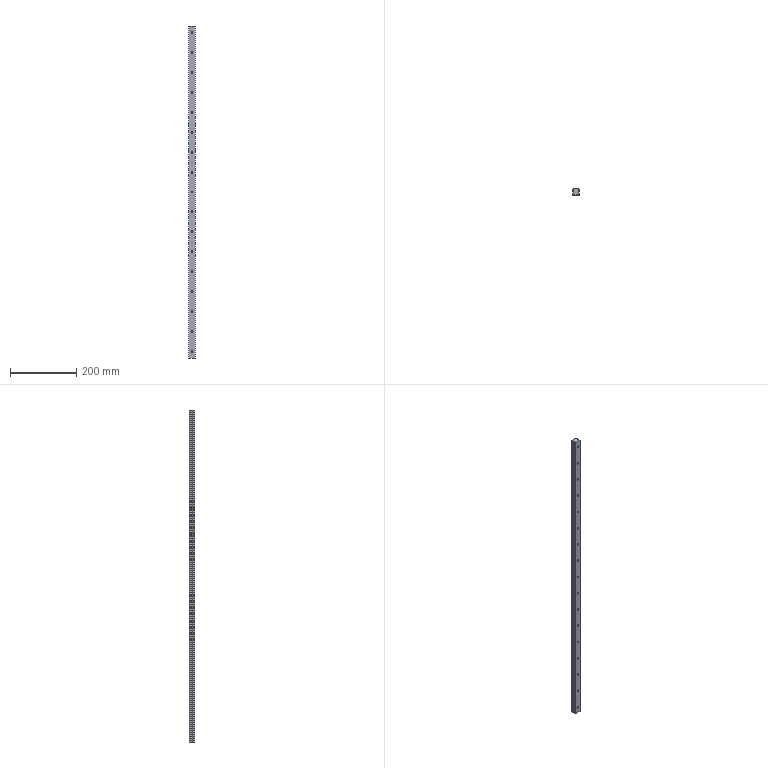Part | SolidWorks | 1 solid | 111 faces | box 20 x 17.5 x 1000 mm | volume 300247 mm3 | cylinder 74 | plane 37 | commonest cylinder face diameters 6 x34 9.5 x34 1.817 x6